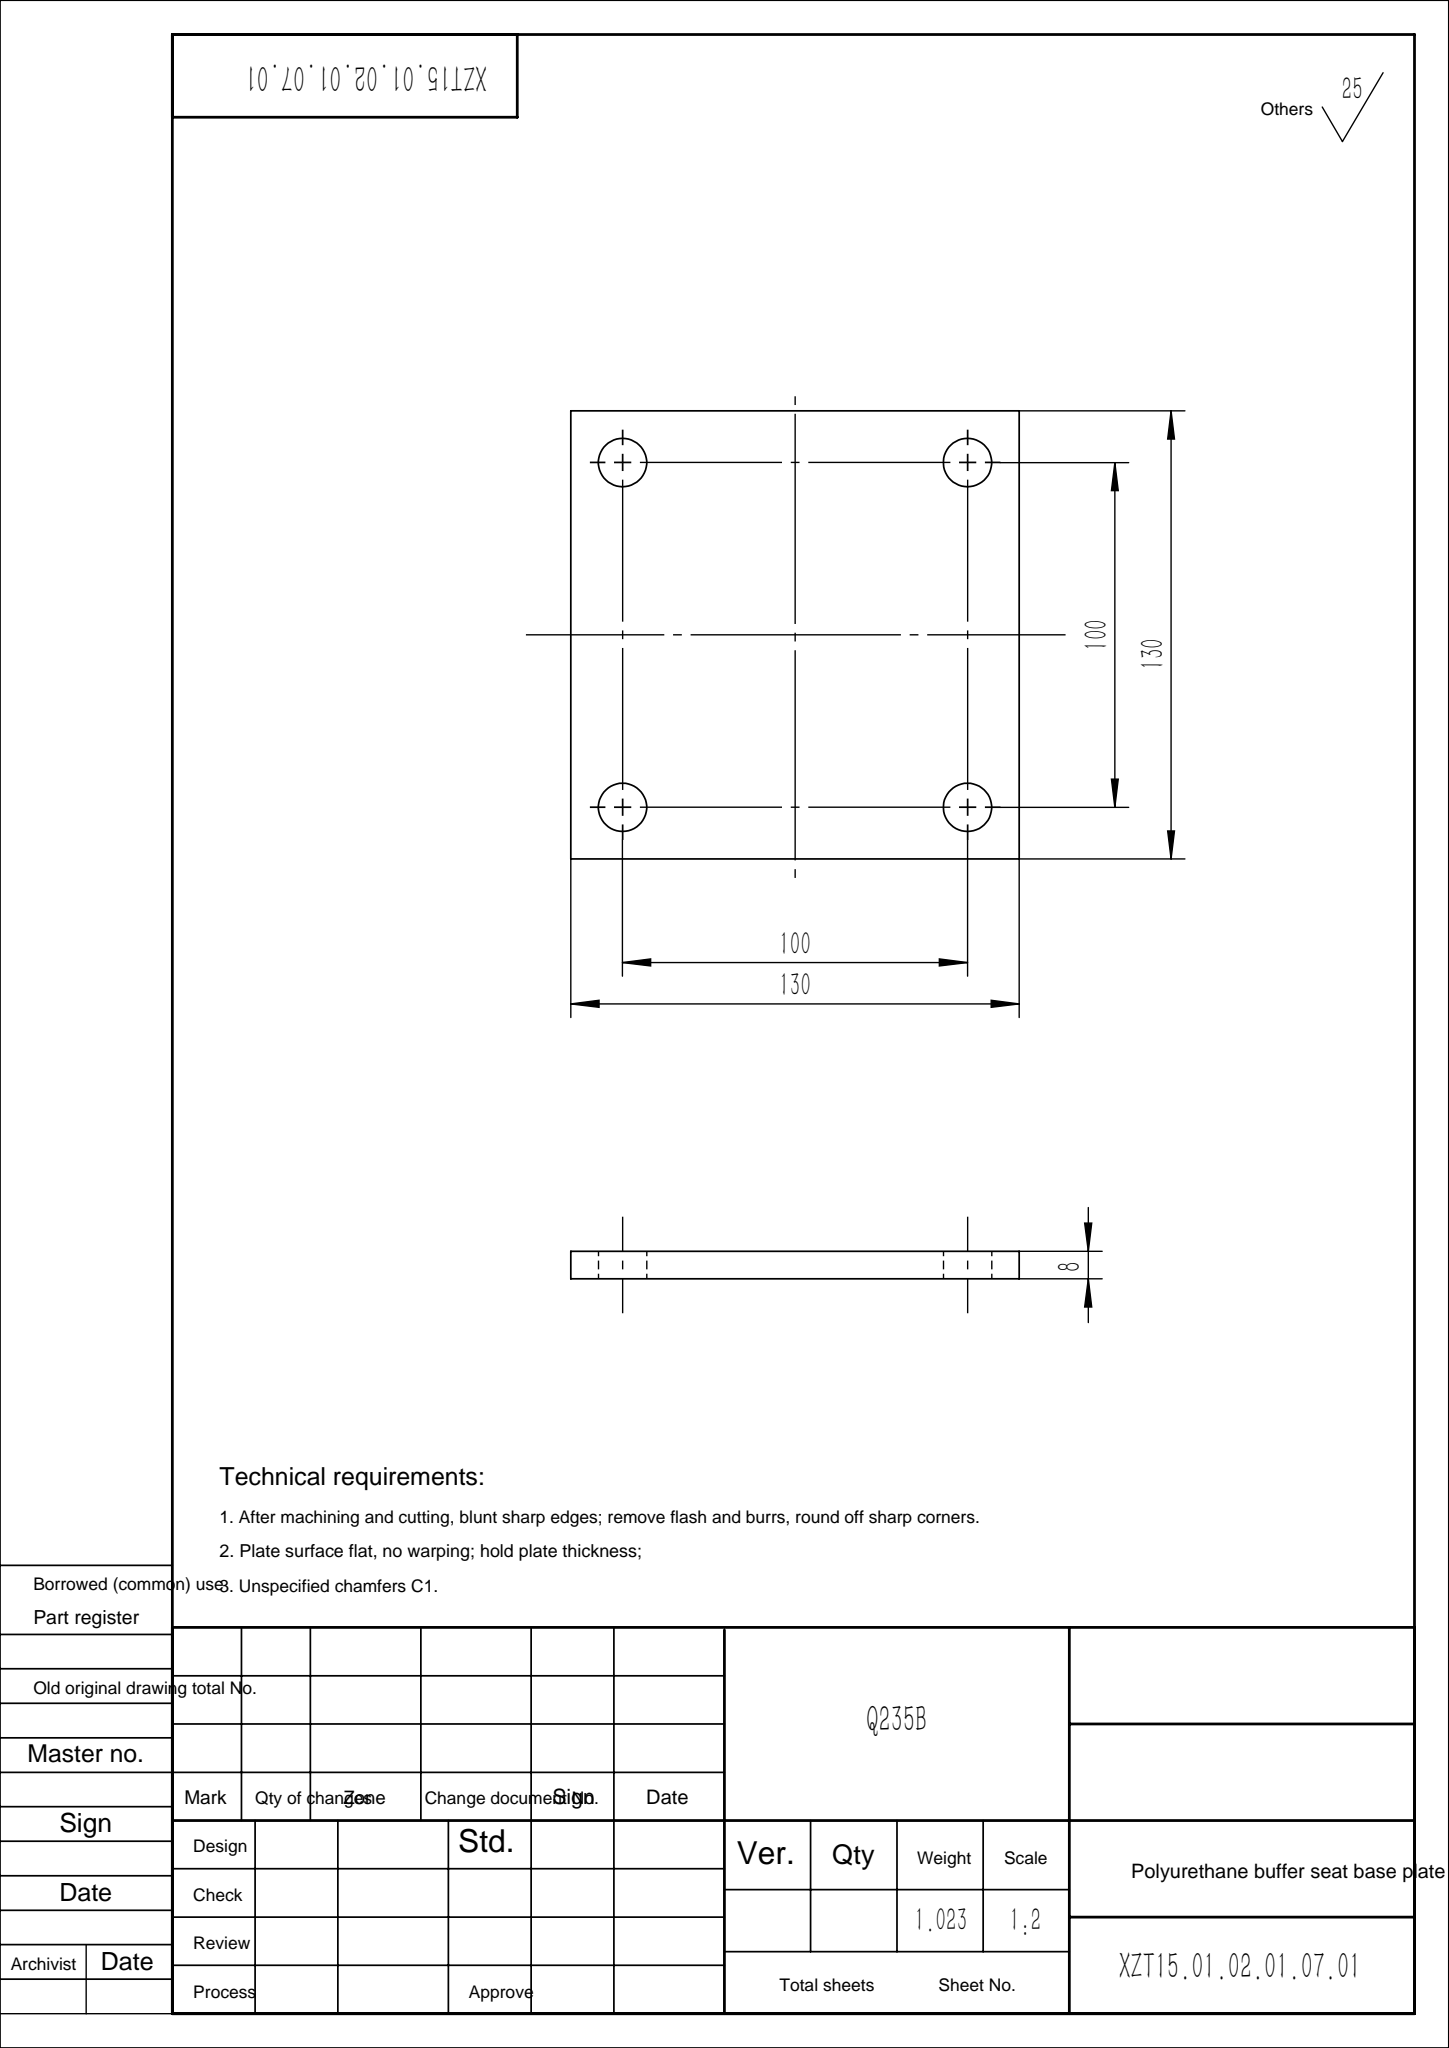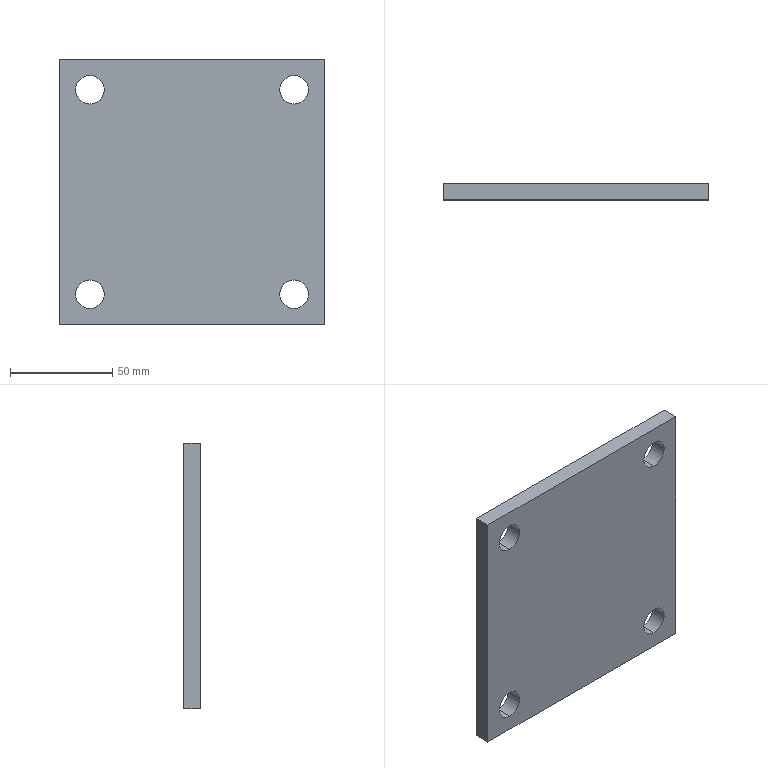Part | SolidWorks | features Chamfer 1, Extrusion 1, Fillet 1, HoleWzd 1 | 1 solid | 14 faces | box 130 x 8 x 130 mm | volume 130274 mm3 | cylinder 8 | plane 6 | commonest cylinder face diameters 14 x8
STEP:
#1=CARTESIAN_POINT('',(-50.,0.,43.));
#2=VERTEX_POINT('',#1);
#3=CARTESIAN_POINT('',(-50.,0.,57.));
#4=VERTEX_POINT('',#3);
#5=CARTESIAN_POINT('',(-50.,0.,50.));
#6=DIRECTION('',(0.,1.,0.));
#7=DIRECTION('',(0.,0.,1.));
#8=AXIS2_PLACEMENT_3D('',#5,#6,#7);
#9=CIRCLE('',#8,7.);
#10=EDGE_CURVE('',#2,#4,#9,.T.);
#11=ORIENTED_EDGE('',*,*,#10,.F.);
#12=CARTESIAN_POINT('',(-50.,8.,43.));
#13=VERTEX_POINT('',#12);
#14=CARTESIAN_POINT('',(-50.,8.,43.));
#15=DIRECTION('',(0.,1.,0.));
#16=VECTOR('',#15,1000.);
#17=LINE('',#14,#16);
#18=EDGE_CURVE('',#2,#13,#17,.T.);
#19=ORIENTED_EDGE('',*,*,#18,.T.);
#20=CARTESIAN_POINT('',(-50.,8.,57.));
#21=VERTEX_POINT('',#20);
#22=CARTESIAN_POINT('',(-50.,8.,50.));
#23=DIRECTION('',(0.,1.,0.));
#24=DIRECTION('',(0.,0.,1.));
#25=AXIS2_PLACEMENT_3D('',#22,#23,#24);
#26=CIRCLE('',#25,7.);
#27=EDGE_CURVE('',#13,#21,#26,.T.);
#28=ORIENTED_EDGE('',*,*,#27,.T.);
#29=CARTESIAN_POINT('',(-50.,8.,57.));
#30=DIRECTION('',(0.,1.,0.));
#31=VECTOR('',#30,1000.);
#32=LINE('',#29,#31);
#33=EDGE_CURVE('',#4,#21,#32,.T.);
#34=ORIENTED_EDGE('',*,*,#33,.F.);
#35=EDGE_LOOP('',(#11,#19,#28,#34));
#36=FACE_OUTER_BOUND('',#35,.T.);
#37=CARTESIAN_POINT('',(-50.,8.,50.));
#38=DIRECTION('',(0.,1.,0.));
#39=DIRECTION('',(0.,0.,1.));
#40=AXIS2_PLACEMENT_3D('',#37,#38,#39);
#41=CYLINDRICAL_SURFACE('',#40,7.);
#42=ADVANCED_FACE('',(#36),#41,.F.);
#43=CARTESIAN_POINT('',(50.,0.,43.));
#44=VERTEX_POINT('',#43);
#45=CARTESIAN_POINT('',(50.,0.,57.));
#46=VERTEX_POINT('',#45);
#47=CARTESIAN_POINT('',(50.,0.,50.));
#48=DIRECTION('',(0.,1.,0.));
#49=DIRECTION('',(0.,0.,1.));
#50=AXIS2_PLACEMENT_3D('',#47,#48,#49);
#51=CIRCLE('',#50,7.);
#52=EDGE_CURVE('',#44,#46,#51,.T.);
#53=ORIENTED_EDGE('',*,*,#52,.F.);
#54=CARTESIAN_POINT('',(50.,8.,43.));
#55=VERTEX_POINT('',#54);
#56=CARTESIAN_POINT('',(50.,8.,43.));
#57=DIRECTION('',(0.,1.,0.));
#58=VECTOR('',#57,1000.);
#59=LINE('',#56,#58);
#60=EDGE_CURVE('',#44,#55,#59,.T.);
#61=ORIENTED_EDGE('',*,*,#60,.T.);
#62=CARTESIAN_POINT('',(50.,8.,57.));
#63=VERTEX_POINT('',#62);
#64=CARTESIAN_POINT('',(50.,8.,50.));
#65=DIRECTION('',(0.,1.,0.));
#66=DIRECTION('',(0.,0.,1.));
#67=AXIS2_PLACEMENT_3D('',#64,#65,#66);
#68=CIRCLE('',#67,7.);
#69=EDGE_CURVE('',#55,#63,#68,.T.);
#70=ORIENTED_EDGE('',*,*,#69,.T.);
#71=CARTESIAN_POINT('',(50.,8.,57.));
#72=DIRECTION('',(0.,1.,0.));
#73=VECTOR('',#72,1000.);
#74=LINE('',#71,#73);
#75=EDGE_CURVE('',#46,#63,#74,.T.);
#76=ORIENTED_EDGE('',*,*,#75,.F.);
#77=EDGE_LOOP('',(#53,#61,#70,#76));
#78=FACE_OUTER_BOUND('',#77,.T.);
#79=CARTESIAN_POINT('',(50.,8.,50.));
#80=DIRECTION('',(0.,1.,0.));
#81=DIRECTION('',(0.,0.,1.));
#82=AXIS2_PLACEMENT_3D('',#79,#80,#81);
#83=CYLINDRICAL_SURFACE('',#82,7.);
#84=ADVANCED_FACE('',(#78),#83,.F.);
#85=CARTESIAN_POINT('',(50.,0.,-57.));
#86=VERTEX_POINT('',#85);
#87=CARTESIAN_POINT('',(50.,0.,-43.));
#88=VERTEX_POINT('',#87);
#89=CARTESIAN_POINT('',(50.,0.,-50.));
#90=DIRECTION('',(0.,1.,0.));
#91=DIRECTION('',(0.,0.,1.));
#92=AXIS2_PLACEMENT_3D('',#89,#90,#91);
#93=CIRCLE('',#92,7.);
#94=EDGE_CURVE('',#86,#88,#93,.T.);
#95=ORIENTED_EDGE('',*,*,#94,.F.);
#96=CARTESIAN_POINT('',(50.,8.,-57.));
#97=VERTEX_POINT('',#96);
#98=CARTESIAN_POINT('',(50.,8.,-57.));
#99=DIRECTION('',(0.,1.,0.));
#100=VECTOR('',#99,1000.);
#101=LINE('',#98,#100);
#102=EDGE_CURVE('',#86,#97,#101,.T.);
#103=ORIENTED_EDGE('',*,*,#102,.T.);
#104=CARTESIAN_POINT('',(50.,8.,-43.));
#105=VERTEX_POINT('',#104);
#106=CARTESIAN_POINT('',(50.,8.,-50.));
#107=DIRECTION('',(0.,1.,0.));
#108=DIRECTION('',(0.,0.,1.));
#109=AXIS2_PLACEMENT_3D('',#106,#107,#108);
#110=CIRCLE('',#109,7.);
#111=EDGE_CURVE('',#97,#105,#110,.T.);
#112=ORIENTED_EDGE('',*,*,#111,.T.);
#113=CARTESIAN_POINT('',(50.,8.,-43.));
#114=DIRECTION('',(0.,1.,0.));
#115=VECTOR('',#114,1000.);
#116=LINE('',#113,#115);
#117=EDGE_CURVE('',#88,#105,#116,.T.);
#118=ORIENTED_EDGE('',*,*,#117,.F.);
#119=EDGE_LOOP('',(#95,#103,#112,#118));
#120=FACE_OUTER_BOUND('',#119,.T.);
#121=CARTESIAN_POINT('',(50.,8.,-50.));
#122=DIRECTION('',(0.,1.,0.));
#123=DIRECTION('',(0.,0.,1.));
#124=AXIS2_PLACEMENT_3D('',#121,#122,#123);
#125=CYLINDRICAL_SURFACE('',#124,7.);
#126=ADVANCED_FACE('',(#120),#125,.F.);
#127=CARTESIAN_POINT('',(-50.,0.,-57.));
#128=VERTEX_POINT('',#127);
#129=CARTESIAN_POINT('',(-50.,0.,-43.));
#130=VERTEX_POINT('',#129);
#131=CARTESIAN_POINT('',(-50.,0.,-50.));
#132=DIRECTION('',(0.,1.,0.));
#133=DIRECTION('',(0.,0.,1.));
#134=AXIS2_PLACEMENT_3D('',#131,#132,#133);
#135=CIRCLE('',#134,7.);
#136=EDGE_CURVE('',#128,#130,#135,.T.);
#137=ORIENTED_EDGE('',*,*,#136,.F.);
#138=CARTESIAN_POINT('',(-50.,8.,-57.));
#139=VERTEX_POINT('',#138);
#140=CARTESIAN_POINT('',(-50.,8.,-57.));
#141=DIRECTION('',(0.,1.,0.));
#142=VECTOR('',#141,1000.);
#143=LINE('',#140,#142);
#144=EDGE_CURVE('',#128,#139,#143,.T.);
#145=ORIENTED_EDGE('',*,*,#144,.T.);
#146=CARTESIAN_POINT('',(-50.,8.,-43.));
#147=VERTEX_POINT('',#146);
#148=CARTESIAN_POINT('',(-50.,8.,-50.));
#149=DIRECTION('',(0.,1.,0.));
#150=DIRECTION('',(0.,0.,1.));
#151=AXIS2_PLACEMENT_3D('',#148,#149,#150);
#152=CIRCLE('',#151,7.);
#153=EDGE_CURVE('',#139,#147,#152,.T.);
#154=ORIENTED_EDGE('',*,*,#153,.T.);
#155=CARTESIAN_POINT('',(-50.,8.,-43.));
#156=DIRECTION('',(0.,1.,0.));
#157=VECTOR('',#156,1000.);
#158=LINE('',#155,#157);
#159=EDGE_CURVE('',#130,#147,#158,.T.);
#160=ORIENTED_EDGE('',*,*,#159,.F.);
#161=EDGE_LOOP('',(#137,#145,#154,#160));
#162=FACE_OUTER_BOUND('',#161,.T.);
#163=CARTESIAN_POINT('',(-50.,8.,-50.));
#164=DIRECTION('',(0.,1.,0.));
#165=DIRECTION('',(0.,0.,1.));
#166=AXIS2_PLACEMENT_3D('',#163,#164,#165);
#167=CYLINDRICAL_SURFACE('',#166,7.);
#168=ADVANCED_FACE('',(#162),#167,.F.);
#169=CARTESIAN_POINT('',(-65.,0.,-65.));
#170=VERTEX_POINT('',#169);
#171=CARTESIAN_POINT('',(-65.,0.,65.));
#172=VERTEX_POINT('',#171);
#173=CARTESIAN_POINT('',(-65.,0.,65.));
#174=DIRECTION('',(0.,0.,1.));
#175=VECTOR('',#174,1000.);
#176=LINE('',#173,#175);
#177=EDGE_CURVE('',#170,#172,#176,.T.);
#178=ORIENTED_EDGE('',*,*,#177,.T.);
#179=CARTESIAN_POINT('',(-65.,8.,65.));
#180=VERTEX_POINT('',#179);
#181=CARTESIAN_POINT('',(-65.,8.,65.));
#182=DIRECTION('',(0.,-1.,0.));
#183=VECTOR('',#182,1000.);
#184=LINE('',#181,#183);
#185=EDGE_CURVE('',#180,#172,#184,.T.);
#186=ORIENTED_EDGE('',*,*,#185,.F.);
#187=CARTESIAN_POINT('',(-65.,8.,-65.));
#188=VERTEX_POINT('',#187);
#189=CARTESIAN_POINT('',(-65.,8.,65.));
#190=DIRECTION('',(0.,0.,1.));
#191=VECTOR('',#190,1000.);
#192=LINE('',#189,#191);
#193=EDGE_CURVE('',#188,#180,#192,.T.);
#194=ORIENTED_EDGE('',*,*,#193,.F.);
#195=CARTESIAN_POINT('',(-65.,8.,-65.));
#196=DIRECTION('',(0.,-1.,0.));
#197=VECTOR('',#196,1000.);
#198=LINE('',#195,#197);
#199=EDGE_CURVE('',#188,#170,#198,.T.);
#200=ORIENTED_EDGE('',*,*,#199,.T.);
#201=EDGE_LOOP('',(#178,#186,#194,#200));
#202=FACE_OUTER_BOUND('',#201,.T.);
#203=CARTESIAN_POINT('',(-65.,8.,65.));
#204=DIRECTION('',(1.,0.,0.));
#205=DIRECTION('',(0.,0.,-1.));
#206=AXIS2_PLACEMENT_3D('',#203,#204,#205);
#207=PLANE('',#206);
#208=ADVANCED_FACE('',(#202),#207,.F.);
#209=CARTESIAN_POINT('',(65.,0.,65.));
#210=VERTEX_POINT('',#209);
#211=CARTESIAN_POINT('',(65.,0.,65.));
#212=DIRECTION('',(1.,0.,0.));
#213=VECTOR('',#212,1000.);
#214=LINE('',#211,#213);
#215=EDGE_CURVE('',#172,#210,#214,.T.);
#216=ORIENTED_EDGE('',*,*,#215,.T.);
#217=CARTESIAN_POINT('',(65.,8.,65.));
#218=VERTEX_POINT('',#217);
#219=CARTESIAN_POINT('',(65.,8.,65.));
#220=DIRECTION('',(0.,-1.,0.));
#221=VECTOR('',#220,1000.);
#222=LINE('',#219,#221);
#223=EDGE_CURVE('',#218,#210,#222,.T.);
#224=ORIENTED_EDGE('',*,*,#223,.F.);
#225=CARTESIAN_POINT('',(65.,8.,65.));
#226=DIRECTION('',(1.,0.,0.));
#227=VECTOR('',#226,1000.);
#228=LINE('',#225,#227);
#229=EDGE_CURVE('',#180,#218,#228,.T.);
#230=ORIENTED_EDGE('',*,*,#229,.F.);
#231=ORIENTED_EDGE('',*,*,#185,.T.);
#232=EDGE_LOOP('',(#216,#224,#230,#231));
#233=FACE_OUTER_BOUND('',#232,.T.);
#234=CARTESIAN_POINT('',(65.,8.,65.));
#235=DIRECTION('',(0.,0.,-1.));
#236=DIRECTION('',(-1.,0.,0.));
#237=AXIS2_PLACEMENT_3D('',#234,#235,#236);
#238=PLANE('',#237);
#239=ADVANCED_FACE('',(#233),#238,.F.);
#240=CARTESIAN_POINT('',(65.,0.,-65.));
#241=VERTEX_POINT('',#240);
#242=CARTESIAN_POINT('',(65.,0.,65.));
#243=DIRECTION('',(0.,0.,-1.));
#244=VECTOR('',#243,1000.);
#245=LINE('',#242,#244);
#246=EDGE_CURVE('',#210,#241,#245,.T.);
#247=ORIENTED_EDGE('',*,*,#246,.T.);
#248=CARTESIAN_POINT('',(65.,8.,-65.));
#249=VERTEX_POINT('',#248);
#250=CARTESIAN_POINT('',(65.,8.,-65.));
#251=DIRECTION('',(0.,-1.,0.));
#252=VECTOR('',#251,1000.);
#253=LINE('',#250,#252);
#254=EDGE_CURVE('',#249,#241,#253,.T.);
#255=ORIENTED_EDGE('',*,*,#254,.F.);
#256=CARTESIAN_POINT('',(65.,8.,65.));
#257=DIRECTION('',(0.,0.,-1.));
#258=VECTOR('',#257,1000.);
#259=LINE('',#256,#258);
#260=EDGE_CURVE('',#218,#249,#259,.T.);
#261=ORIENTED_EDGE('',*,*,#260,.F.);
#262=ORIENTED_EDGE('',*,*,#223,.T.);
#263=EDGE_LOOP('',(#247,#255,#261,#262));
#264=FACE_OUTER_BOUND('',#263,.T.);
#265=CARTESIAN_POINT('',(65.,8.,65.));
#266=DIRECTION('',(-1.,0.,0.));
#267=DIRECTION('',(0.,0.,1.));
#268=AXIS2_PLACEMENT_3D('',#265,#266,#267);
#269=PLANE('',#268);
#270=ADVANCED_FACE('',(#264),#269,.F.);
#271=CARTESIAN_POINT('',(65.,0.,-65.));
#272=DIRECTION('',(-1.,0.,0.));
#273=VECTOR('',#272,1000.);
#274=LINE('',#271,#273);
#275=EDGE_CURVE('',#241,#170,#274,.T.);
#276=ORIENTED_EDGE('',*,*,#275,.T.);
#277=ORIENTED_EDGE('',*,*,#199,.F.);
#278=CARTESIAN_POINT('',(65.,8.,-65.));
#279=DIRECTION('',(-1.,0.,0.));
#280=VECTOR('',#279,1000.);
#281=LINE('',#278,#280);
#282=EDGE_CURVE('',#249,#188,#281,.T.);
#283=ORIENTED_EDGE('',*,*,#282,.F.);
#284=ORIENTED_EDGE('',*,*,#254,.T.);
#285=EDGE_LOOP('',(#276,#277,#283,#284));
#286=FACE_OUTER_BOUND('',#285,.T.);
#287=CARTESIAN_POINT('',(65.,8.,-65.));
#288=DIRECTION('',(0.,0.,1.));
#289=DIRECTION('',(1.,0.,0.));
#290=AXIS2_PLACEMENT_3D('',#287,#288,#289);
#291=PLANE('',#290);
#292=ADVANCED_FACE('',(#286),#291,.F.);
#293=CARTESIAN_POINT('',(-50.,8.,50.));
#294=DIRECTION('',(0.,1.,0.));
#295=DIRECTION('',(0.,0.,1.));
#296=AXIS2_PLACEMENT_3D('',#293,#294,#295);
#297=CIRCLE('',#296,7.);
#298=EDGE_CURVE('',#21,#13,#297,.T.);
#299=ORIENTED_EDGE('',*,*,#298,.F.);
#300=ORIENTED_EDGE('',*,*,#27,.F.);
#301=EDGE_LOOP('',(#299,#300));
#302=FACE_BOUND('',#301,.T.);
#303=CARTESIAN_POINT('',(50.,8.,50.));
#304=DIRECTION('',(0.,1.,0.));
#305=DIRECTION('',(0.,0.,1.));
#306=AXIS2_PLACEMENT_3D('',#303,#304,#305);
#307=CIRCLE('',#306,7.);
#308=EDGE_CURVE('',#63,#55,#307,.T.);
#309=ORIENTED_EDGE('',*,*,#308,.F.);
#310=ORIENTED_EDGE('',*,*,#69,.F.);
#311=EDGE_LOOP('',(#309,#310));
#312=FACE_BOUND('',#311,.T.);
#313=CARTESIAN_POINT('',(50.,8.,-50.));
#314=DIRECTION('',(0.,1.,0.));
#315=DIRECTION('',(0.,0.,1.));
#316=AXIS2_PLACEMENT_3D('',#313,#314,#315);
#317=CIRCLE('',#316,7.);
#318=EDGE_CURVE('',#105,#97,#317,.T.);
#319=ORIENTED_EDGE('',*,*,#318,.F.);
#320=ORIENTED_EDGE('',*,*,#111,.F.);
#321=EDGE_LOOP('',(#319,#320));
#322=FACE_BOUND('',#321,.T.);
#323=CARTESIAN_POINT('',(-50.,8.,-50.));
#324=DIRECTION('',(0.,1.,0.));
#325=DIRECTION('',(0.,0.,1.));
#326=AXIS2_PLACEMENT_3D('',#323,#324,#325);
#327=CIRCLE('',#326,7.);
#328=EDGE_CURVE('',#147,#139,#327,.T.);
#329=ORIENTED_EDGE('',*,*,#328,.F.);
#330=ORIENTED_EDGE('',*,*,#153,.F.);
#331=EDGE_LOOP('',(#329,#330));
#332=FACE_BOUND('',#331,.T.);
#333=ORIENTED_EDGE('',*,*,#193,.T.);
#334=ORIENTED_EDGE('',*,*,#229,.T.);
#335=ORIENTED_EDGE('',*,*,#260,.T.);
#336=ORIENTED_EDGE('',*,*,#282,.T.);
#337=EDGE_LOOP('',(#333,#334,#335,#336));
#338=FACE_OUTER_BOUND('',#337,.T.);
#339=CARTESIAN_POINT('',(0.,8.,0.));
#340=DIRECTION('',(0.,1.,0.));
#341=DIRECTION('',(0.,0.,1.));
#342=AXIS2_PLACEMENT_3D('',#339,#340,#341);
#343=PLANE('',#342);
#344=ADVANCED_FACE('',(#302,#312,#322,#332,#338),#343,.T.);
#345=CARTESIAN_POINT('',(-50.,0.,50.));
#346=DIRECTION('',(0.,1.,0.));
#347=DIRECTION('',(0.,0.,1.));
#348=AXIS2_PLACEMENT_3D('',#345,#346,#347);
#349=CIRCLE('',#348,7.);
#350=EDGE_CURVE('',#4,#2,#349,.T.);
#351=ORIENTED_EDGE('',*,*,#350,.T.);
#352=ORIENTED_EDGE('',*,*,#10,.T.);
#353=EDGE_LOOP('',(#351,#352));
#354=FACE_BOUND('',#353,.T.);
#355=CARTESIAN_POINT('',(50.,0.,50.));
#356=DIRECTION('',(0.,1.,0.));
#357=DIRECTION('',(0.,0.,1.));
#358=AXIS2_PLACEMENT_3D('',#355,#356,#357);
#359=CIRCLE('',#358,7.);
#360=EDGE_CURVE('',#46,#44,#359,.T.);
#361=ORIENTED_EDGE('',*,*,#360,.T.);
#362=ORIENTED_EDGE('',*,*,#52,.T.);
#363=EDGE_LOOP('',(#361,#362));
#364=FACE_BOUND('',#363,.T.);
#365=CARTESIAN_POINT('',(50.,0.,-50.));
#366=DIRECTION('',(0.,1.,0.));
#367=DIRECTION('',(0.,0.,1.));
#368=AXIS2_PLACEMENT_3D('',#365,#366,#367);
#369=CIRCLE('',#368,7.);
#370=EDGE_CURVE('',#88,#86,#369,.T.);
#371=ORIENTED_EDGE('',*,*,#370,.T.);
#372=ORIENTED_EDGE('',*,*,#94,.T.);
#373=EDGE_LOOP('',(#371,#372));
#374=FACE_BOUND('',#373,.T.);
#375=CARTESIAN_POINT('',(-50.,0.,-50.));
#376=DIRECTION('',(0.,1.,0.));
#377=DIRECTION('',(0.,0.,1.));
#378=AXIS2_PLACEMENT_3D('',#375,#376,#377);
#379=CIRCLE('',#378,7.);
#380=EDGE_CURVE('',#130,#128,#379,.T.);
#381=ORIENTED_EDGE('',*,*,#380,.T.);
#382=ORIENTED_EDGE('',*,*,#136,.T.);
#383=EDGE_LOOP('',(#381,#382));
#384=FACE_BOUND('',#383,.T.);
#385=ORIENTED_EDGE('',*,*,#177,.F.);
#386=ORIENTED_EDGE('',*,*,#275,.F.);
#387=ORIENTED_EDGE('',*,*,#246,.F.);
#388=ORIENTED_EDGE('',*,*,#215,.F.);
#389=EDGE_LOOP('',(#385,#386,#387,#388));
#390=FACE_OUTER_BOUND('',#389,.T.);
#391=CARTESIAN_POINT('',(0.,0.,0.));
#392=DIRECTION('',(0.,1.,0.));
#393=DIRECTION('',(0.,0.,1.));
#394=AXIS2_PLACEMENT_3D('',#391,#392,#393);
#395=PLANE('',#394);
#396=ADVANCED_FACE('',(#354,#364,#374,#384,#390),#395,.F.);
#397=ORIENTED_EDGE('',*,*,#144,.F.);
#398=ORIENTED_EDGE('',*,*,#380,.F.);
#399=ORIENTED_EDGE('',*,*,#159,.T.);
#400=ORIENTED_EDGE('',*,*,#328,.T.);
#401=EDGE_LOOP('',(#397,#398,#399,#400));
#402=FACE_OUTER_BOUND('',#401,.T.);
#403=CARTESIAN_POINT('',(-50.,8.,-50.));
#404=DIRECTION('',(0.,1.,0.));
#405=DIRECTION('',(0.,0.,1.));
#406=AXIS2_PLACEMENT_3D('',#403,#404,#405);
#407=CYLINDRICAL_SURFACE('',#406,7.);
#408=ADVANCED_FACE('',(#402),#407,.F.);
#409=ORIENTED_EDGE('',*,*,#102,.F.);
#410=ORIENTED_EDGE('',*,*,#370,.F.);
#411=ORIENTED_EDGE('',*,*,#117,.T.);
#412=ORIENTED_EDGE('',*,*,#318,.T.);
#413=EDGE_LOOP('',(#409,#410,#411,#412));
#414=FACE_OUTER_BOUND('',#413,.T.);
#415=CARTESIAN_POINT('',(50.,8.,-50.));
#416=DIRECTION('',(0.,1.,0.));
#417=DIRECTION('',(0.,0.,1.));
#418=AXIS2_PLACEMENT_3D('',#415,#416,#417);
#419=CYLINDRICAL_SURFACE('',#418,7.);
#420=ADVANCED_FACE('',(#414),#419,.F.);
#421=ORIENTED_EDGE('',*,*,#60,.F.);
#422=ORIENTED_EDGE('',*,*,#360,.F.);
#423=ORIENTED_EDGE('',*,*,#75,.T.);
#424=ORIENTED_EDGE('',*,*,#308,.T.);
#425=EDGE_LOOP('',(#421,#422,#423,#424));
#426=FACE_OUTER_BOUND('',#425,.T.);
#427=CARTESIAN_POINT('',(50.,8.,50.));
#428=DIRECTION('',(0.,1.,0.));
#429=DIRECTION('',(0.,0.,1.));
#430=AXIS2_PLACEMENT_3D('',#427,#428,#429);
#431=CYLINDRICAL_SURFACE('',#430,7.);
#432=ADVANCED_FACE('',(#426),#431,.F.);
#433=ORIENTED_EDGE('',*,*,#18,.F.);
#434=ORIENTED_EDGE('',*,*,#350,.F.);
#435=ORIENTED_EDGE('',*,*,#33,.T.);
#436=ORIENTED_EDGE('',*,*,#298,.T.);
#437=EDGE_LOOP('',(#433,#434,#435,#436));
#438=FACE_OUTER_BOUND('',#437,.T.);
#439=CARTESIAN_POINT('',(-50.,8.,50.));
#440=DIRECTION('',(0.,1.,0.));
#441=DIRECTION('',(0.,0.,1.));
#442=AXIS2_PLACEMENT_3D('',#439,#440,#441);
#443=CYLINDRICAL_SURFACE('',#442,7.);
#444=ADVANCED_FACE('',(#438),#443,.F.);
#445=CLOSED_SHELL('',(#42,#84,#126,#168,#208,#239,#270,#292,#344,#396,#408,#420,#432,#444));
#446=MANIFOLD_SOLID_BREP('',#445);
#447=CARTESIAN_POINT('',(0.,0.,0.));
#448=DIRECTION('',(0.,0.,1.));
#449=DIRECTION('',(1.,0.,0.));
#450=AXIS2_PLACEMENT_3D('',#447,#448,#449);
#451=(LENGTH_UNIT()NAMED_UNIT(*)SI_UNIT(.MILLI.,.METRE.));
#452=UNCERTAINTY_MEASURE_WITH_UNIT(LENGTH_MEASURE(0.00001),#451,'','');
#453=(NAMED_UNIT(*)PLANE_ANGLE_UNIT()SI_UNIT($,.RADIAN.));
#454=(NAMED_UNIT(*)SI_UNIT($,.STERADIAN.)SOLID_ANGLE_UNIT());
#455=(GEOMETRIC_REPRESENTATION_CONTEXT(3)GLOBAL_UNCERTAINTY_ASSIGNED_CONTEXT((#452))GLOBAL_UNIT_ASSIGNED_CONTEXT((#451,#453,#454))REPRESENTATION_CONTEXT('',''));
#456=ADVANCED_BREP_SHAPE_REPRESENTATION('',(#446,#450),#455);